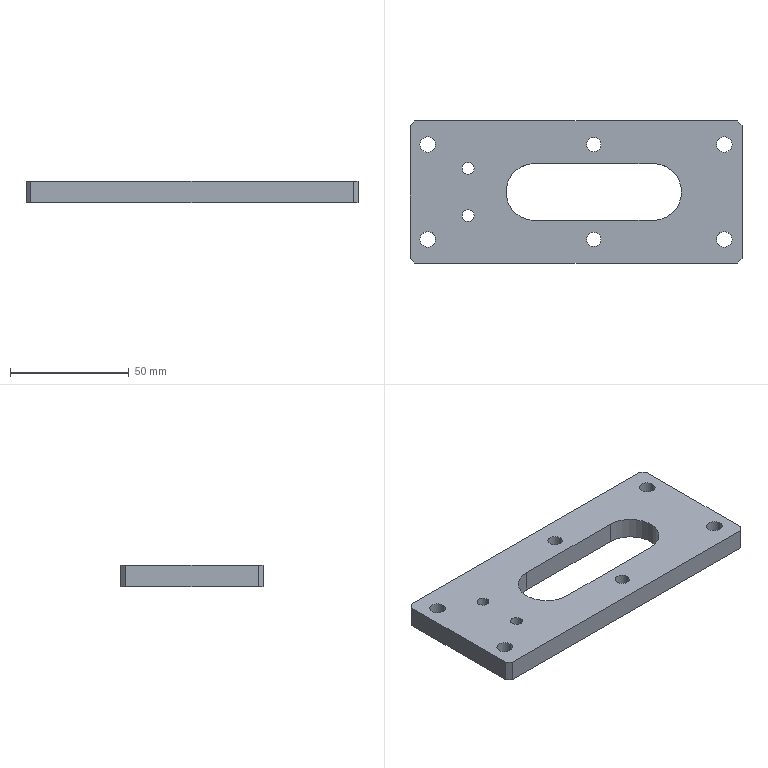Part | STEP file | TNSN20-Y20-F22-Part-14-1 | 1 solid | 30 faces | box 140 x 60 x 9 mm | volume 58562 mm3 | cylinder 18 | plane 12 | commonest cylinder face diameters 6.6 x8 5 x4 6 x4 24 x2
STEP:
#1=CARTESIAN_POINT('',(14042.245,13730.046,0.));
#2=VERTEX_POINT('',#1);
#3=CARTESIAN_POINT('',(14037.245,13730.046,0.));
#4=VERTEX_POINT('',#3);
#5=CARTESIAN_POINT('',(14039.745,13730.046,0.));
#6=DIRECTION('',(0.,0.,-1.));
#7=DIRECTION('',(1.,0.,0.));
#8=AXIS2_PLACEMENT_3D('',#5,#6,#7);
#9=CIRCLE('',#8,2.5);
#10=EDGE_CURVE('',#2,#4,#9,.T.);
#11=ORIENTED_EDGE('',*,*,#10,.T.);
#12=CARTESIAN_POINT('',(14037.245,13730.046,9.));
#13=VERTEX_POINT('',#12);
#14=CARTESIAN_POINT('',(14037.245,13730.046,0.));
#15=DIRECTION('',(0.,0.,1.));
#16=VECTOR('',#15,1000.);
#17=LINE('',#14,#16);
#18=EDGE_CURVE('',#4,#13,#17,.T.);
#19=ORIENTED_EDGE('',*,*,#18,.T.);
#20=CARTESIAN_POINT('',(14042.245,13730.046,9.));
#21=VERTEX_POINT('',#20);
#22=CARTESIAN_POINT('',(14039.745,13730.046,9.));
#23=DIRECTION('',(0.,0.,1.));
#24=DIRECTION('',(-1.,0.,0.));
#25=AXIS2_PLACEMENT_3D('',#22,#23,#24);
#26=CIRCLE('',#25,2.5);
#27=EDGE_CURVE('',#13,#21,#26,.T.);
#28=ORIENTED_EDGE('',*,*,#27,.T.);
#29=CARTESIAN_POINT('',(14042.245,13730.046,0.));
#30=DIRECTION('',(0.,0.,1.));
#31=VECTOR('',#30,1000.);
#32=LINE('',#29,#31);
#33=EDGE_CURVE('',#2,#21,#32,.T.);
#34=ORIENTED_EDGE('',*,*,#33,.F.);
#35=EDGE_LOOP('',(#11,#19,#28,#34));
#36=FACE_OUTER_BOUND('',#35,.T.);
#37=CARTESIAN_POINT('',(14039.745,13730.046,0.));
#38=DIRECTION('',(0.,0.,1.));
#39=DIRECTION('',(1.,0.,0.));
#40=AXIS2_PLACEMENT_3D('',#37,#38,#39);
#41=CYLINDRICAL_SURFACE('',#40,2.5);
#42=ADVANCED_FACE('',(#36),#41,.F.);
#43=CARTESIAN_POINT('',(14042.245,13710.046,0.));
#44=VERTEX_POINT('',#43);
#45=CARTESIAN_POINT('',(14037.245,13710.046,0.));
#46=VERTEX_POINT('',#45);
#47=CARTESIAN_POINT('',(14039.745,13710.046,0.));
#48=DIRECTION('',(0.,0.,-1.));
#49=DIRECTION('',(1.,0.,0.));
#50=AXIS2_PLACEMENT_3D('',#47,#48,#49);
#51=CIRCLE('',#50,2.5);
#52=EDGE_CURVE('',#44,#46,#51,.T.);
#53=ORIENTED_EDGE('',*,*,#52,.T.);
#54=CARTESIAN_POINT('',(14037.245,13710.046,9.));
#55=VERTEX_POINT('',#54);
#56=CARTESIAN_POINT('',(14037.245,13710.046,0.));
#57=DIRECTION('',(0.,0.,1.));
#58=VECTOR('',#57,1000.);
#59=LINE('',#56,#58);
#60=EDGE_CURVE('',#46,#55,#59,.T.);
#61=ORIENTED_EDGE('',*,*,#60,.T.);
#62=CARTESIAN_POINT('',(14042.245,13710.046,9.));
#63=VERTEX_POINT('',#62);
#64=CARTESIAN_POINT('',(14039.745,13710.046,9.));
#65=DIRECTION('',(0.,0.,1.));
#66=DIRECTION('',(-1.,0.,0.));
#67=AXIS2_PLACEMENT_3D('',#64,#65,#66);
#68=CIRCLE('',#67,2.5);
#69=EDGE_CURVE('',#55,#63,#68,.T.);
#70=ORIENTED_EDGE('',*,*,#69,.T.);
#71=CARTESIAN_POINT('',(14042.245,13710.046,0.));
#72=DIRECTION('',(0.,0.,1.));
#73=VECTOR('',#72,1000.);
#74=LINE('',#71,#73);
#75=EDGE_CURVE('',#44,#63,#74,.T.);
#76=ORIENTED_EDGE('',*,*,#75,.F.);
#77=EDGE_LOOP('',(#53,#61,#70,#76));
#78=FACE_OUTER_BOUND('',#77,.T.);
#79=CARTESIAN_POINT('',(14039.745,13710.046,0.));
#80=DIRECTION('',(0.,0.,1.));
#81=DIRECTION('',(1.,0.,0.));
#82=AXIS2_PLACEMENT_3D('',#79,#80,#81);
#83=CYLINDRICAL_SURFACE('',#82,2.5);
#84=ADVANCED_FACE('',(#78),#83,.F.);
#85=CARTESIAN_POINT('',(14095.745,13740.046,0.));
#86=VERTEX_POINT('',#85);
#87=CARTESIAN_POINT('',(14089.745,13740.046,0.));
#88=VERTEX_POINT('',#87);
#89=CARTESIAN_POINT('',(14092.745,13740.046,0.));
#90=DIRECTION('',(0.,0.,-1.));
#91=DIRECTION('',(-1.,0.,0.));
#92=AXIS2_PLACEMENT_3D('',#89,#90,#91);
#93=CIRCLE('',#92,3.);
#94=EDGE_CURVE('',#86,#88,#93,.T.);
#95=ORIENTED_EDGE('',*,*,#94,.T.);
#96=CARTESIAN_POINT('',(14089.745,13740.046,9.));
#97=VERTEX_POINT('',#96);
#98=CARTESIAN_POINT('',(14089.745,13740.046,0.));
#99=DIRECTION('',(0.,0.,1.));
#100=VECTOR('',#99,1000.);
#101=LINE('',#98,#100);
#102=EDGE_CURVE('',#88,#97,#101,.T.);
#103=ORIENTED_EDGE('',*,*,#102,.T.);
#104=CARTESIAN_POINT('',(14095.745,13740.046,9.));
#105=VERTEX_POINT('',#104);
#106=CARTESIAN_POINT('',(14092.745,13740.046,9.));
#107=DIRECTION('',(0.,0.,-1.));
#108=DIRECTION('',(-1.,0.,0.));
#109=AXIS2_PLACEMENT_3D('',#106,#107,#108);
#110=CIRCLE('',#109,3.);
#111=EDGE_CURVE('',#105,#97,#110,.T.);
#112=ORIENTED_EDGE('',*,*,#111,.F.);
#113=CARTESIAN_POINT('',(14095.745,13740.046,0.));
#114=DIRECTION('',(0.,0.,1.));
#115=VECTOR('',#114,1000.);
#116=LINE('',#113,#115);
#117=EDGE_CURVE('',#86,#105,#116,.T.);
#118=ORIENTED_EDGE('',*,*,#117,.F.);
#119=EDGE_LOOP('',(#95,#103,#112,#118));
#120=FACE_OUTER_BOUND('',#119,.T.);
#121=CARTESIAN_POINT('',(14092.745,13740.046,0.));
#122=DIRECTION('',(0.,0.,1.));
#123=DIRECTION('',(1.,0.,0.));
#124=AXIS2_PLACEMENT_3D('',#121,#122,#123);
#125=CYLINDRICAL_SURFACE('',#124,3.);
#126=ADVANCED_FACE('',(#120),#125,.F.);
#127=CARTESIAN_POINT('',(14095.745,13700.046,0.));
#128=VERTEX_POINT('',#127);
#129=CARTESIAN_POINT('',(14089.745,13700.046,0.));
#130=VERTEX_POINT('',#129);
#131=CARTESIAN_POINT('',(14092.745,13700.046,0.));
#132=DIRECTION('',(0.,0.,-1.));
#133=DIRECTION('',(-1.,0.,0.));
#134=AXIS2_PLACEMENT_3D('',#131,#132,#133);
#135=CIRCLE('',#134,3.);
#136=EDGE_CURVE('',#128,#130,#135,.T.);
#137=ORIENTED_EDGE('',*,*,#136,.T.);
#138=CARTESIAN_POINT('',(14089.745,13700.046,9.));
#139=VERTEX_POINT('',#138);
#140=CARTESIAN_POINT('',(14089.745,13700.046,0.));
#141=DIRECTION('',(0.,0.,1.));
#142=VECTOR('',#141,1000.);
#143=LINE('',#140,#142);
#144=EDGE_CURVE('',#130,#139,#143,.T.);
#145=ORIENTED_EDGE('',*,*,#144,.T.);
#146=CARTESIAN_POINT('',(14095.745,13700.046,9.));
#147=VERTEX_POINT('',#146);
#148=CARTESIAN_POINT('',(14092.745,13700.046,9.));
#149=DIRECTION('',(0.,0.,-1.));
#150=DIRECTION('',(-1.,0.,0.));
#151=AXIS2_PLACEMENT_3D('',#148,#149,#150);
#152=CIRCLE('',#151,3.);
#153=EDGE_CURVE('',#147,#139,#152,.T.);
#154=ORIENTED_EDGE('',*,*,#153,.F.);
#155=CARTESIAN_POINT('',(14095.745,13700.046,0.));
#156=DIRECTION('',(0.,0.,1.));
#157=VECTOR('',#156,1000.);
#158=LINE('',#155,#157);
#159=EDGE_CURVE('',#128,#147,#158,.T.);
#160=ORIENTED_EDGE('',*,*,#159,.F.);
#161=EDGE_LOOP('',(#137,#145,#154,#160));
#162=FACE_OUTER_BOUND('',#161,.T.);
#163=CARTESIAN_POINT('',(14092.745,13700.046,0.));
#164=DIRECTION('',(0.,0.,1.));
#165=DIRECTION('',(1.,0.,0.));
#166=AXIS2_PLACEMENT_3D('',#163,#164,#165);
#167=CYLINDRICAL_SURFACE('',#166,3.);
#168=ADVANCED_FACE('',(#162),#167,.F.);
#169=CARTESIAN_POINT('',(14019.445,13700.046,9.));
#170=VERTEX_POINT('',#169);
#171=CARTESIAN_POINT('',(14026.045,13700.046,9.));
#172=VERTEX_POINT('',#171);
#173=CARTESIAN_POINT('',(14022.745,13700.046,9.));
#174=DIRECTION('',(0.,0.,1.));
#175=DIRECTION('',(1.,0.,0.));
#176=AXIS2_PLACEMENT_3D('',#173,#174,#175);
#177=CIRCLE('',#176,3.3);
#178=EDGE_CURVE('',#170,#172,#177,.T.);
#179=ORIENTED_EDGE('',*,*,#178,.T.);
#180=CARTESIAN_POINT('',(14026.045,13700.046,0.));
#181=VERTEX_POINT('',#180);
#182=CARTESIAN_POINT('',(14026.045,13700.046,4.5));
#183=DIRECTION('',(0.,0.,-1.));
#184=VECTOR('',#183,1000.);
#185=LINE('',#182,#184);
#186=EDGE_CURVE('',#172,#181,#185,.T.);
#187=ORIENTED_EDGE('',*,*,#186,.T.);
#188=CARTESIAN_POINT('',(14019.445,13700.046,0.));
#189=VERTEX_POINT('',#188);
#190=CARTESIAN_POINT('',(14022.745,13700.046,0.));
#191=DIRECTION('',(0.,0.,1.));
#192=DIRECTION('',(1.,0.,0.));
#193=AXIS2_PLACEMENT_3D('',#190,#191,#192);
#194=CIRCLE('',#193,3.3);
#195=EDGE_CURVE('',#189,#181,#194,.T.);
#196=ORIENTED_EDGE('',*,*,#195,.F.);
#197=CARTESIAN_POINT('',(14019.445,13700.046,4.5));
#198=DIRECTION('',(0.,0.,-1.));
#199=VECTOR('',#198,1000.);
#200=LINE('',#197,#199);
#201=EDGE_CURVE('',#170,#189,#200,.T.);
#202=ORIENTED_EDGE('',*,*,#201,.F.);
#203=EDGE_LOOP('',(#179,#187,#196,#202));
#204=FACE_OUTER_BOUND('',#203,.T.);
#205=CARTESIAN_POINT('',(14022.745,13700.046,4.5));
#206=DIRECTION('',(0.,0.,-1.));
#207=DIRECTION('',(-1.,0.,0.));
#208=AXIS2_PLACEMENT_3D('',#205,#206,#207);
#209=CYLINDRICAL_SURFACE('',#208,3.3);
#210=ADVANCED_FACE('',(#204),#209,.F.);
#211=CARTESIAN_POINT('',(14019.445,13740.046,9.));
#212=VERTEX_POINT('',#211);
#213=CARTESIAN_POINT('',(14026.045,13740.046,9.));
#214=VERTEX_POINT('',#213);
#215=CARTESIAN_POINT('',(14022.745,13740.046,9.));
#216=DIRECTION('',(0.,0.,1.));
#217=DIRECTION('',(1.,0.,0.));
#218=AXIS2_PLACEMENT_3D('',#215,#216,#217);
#219=CIRCLE('',#218,3.3);
#220=EDGE_CURVE('',#212,#214,#219,.T.);
#221=ORIENTED_EDGE('',*,*,#220,.T.);
#222=CARTESIAN_POINT('',(14026.045,13740.046,0.));
#223=VERTEX_POINT('',#222);
#224=CARTESIAN_POINT('',(14026.045,13740.046,4.5));
#225=DIRECTION('',(0.,0.,-1.));
#226=VECTOR('',#225,1000.);
#227=LINE('',#224,#226);
#228=EDGE_CURVE('',#214,#223,#227,.T.);
#229=ORIENTED_EDGE('',*,*,#228,.T.);
#230=CARTESIAN_POINT('',(14019.445,13740.046,0.));
#231=VERTEX_POINT('',#230);
#232=CARTESIAN_POINT('',(14022.745,13740.046,0.));
#233=DIRECTION('',(0.,0.,1.));
#234=DIRECTION('',(1.,0.,0.));
#235=AXIS2_PLACEMENT_3D('',#232,#233,#234);
#236=CIRCLE('',#235,3.3);
#237=EDGE_CURVE('',#231,#223,#236,.T.);
#238=ORIENTED_EDGE('',*,*,#237,.F.);
#239=CARTESIAN_POINT('',(14019.445,13740.046,4.5));
#240=DIRECTION('',(0.,0.,-1.));
#241=VECTOR('',#240,1000.);
#242=LINE('',#239,#241);
#243=EDGE_CURVE('',#212,#231,#242,.T.);
#244=ORIENTED_EDGE('',*,*,#243,.F.);
#245=EDGE_LOOP('',(#221,#229,#238,#244));
#246=FACE_OUTER_BOUND('',#245,.T.);
#247=CARTESIAN_POINT('',(14022.745,13740.046,4.5));
#248=DIRECTION('',(0.,0.,-1.));
#249=DIRECTION('',(-1.,0.,0.));
#250=AXIS2_PLACEMENT_3D('',#247,#248,#249);
#251=CYLINDRICAL_SURFACE('',#250,3.3);
#252=ADVANCED_FACE('',(#246),#251,.F.);
#253=CARTESIAN_POINT('',(14144.445,13700.046,9.));
#254=VERTEX_POINT('',#253);
#255=CARTESIAN_POINT('',(14151.045,13700.046,9.));
#256=VERTEX_POINT('',#255);
#257=CARTESIAN_POINT('',(14147.745,13700.046,9.));
#258=DIRECTION('',(0.,0.,1.));
#259=DIRECTION('',(1.,0.,0.));
#260=AXIS2_PLACEMENT_3D('',#257,#258,#259);
#261=CIRCLE('',#260,3.3);
#262=EDGE_CURVE('',#254,#256,#261,.T.);
#263=ORIENTED_EDGE('',*,*,#262,.T.);
#264=CARTESIAN_POINT('',(14151.045,13700.046,0.));
#265=VERTEX_POINT('',#264);
#266=CARTESIAN_POINT('',(14151.045,13700.046,4.5));
#267=DIRECTION('',(0.,0.,-1.));
#268=VECTOR('',#267,1000.);
#269=LINE('',#266,#268);
#270=EDGE_CURVE('',#256,#265,#269,.T.);
#271=ORIENTED_EDGE('',*,*,#270,.T.);
#272=CARTESIAN_POINT('',(14144.445,13700.046,0.));
#273=VERTEX_POINT('',#272);
#274=CARTESIAN_POINT('',(14147.745,13700.046,0.));
#275=DIRECTION('',(0.,0.,1.));
#276=DIRECTION('',(1.,0.,0.));
#277=AXIS2_PLACEMENT_3D('',#274,#275,#276);
#278=CIRCLE('',#277,3.3);
#279=EDGE_CURVE('',#273,#265,#278,.T.);
#280=ORIENTED_EDGE('',*,*,#279,.F.);
#281=CARTESIAN_POINT('',(14144.445,13700.046,4.5));
#282=DIRECTION('',(0.,0.,-1.));
#283=VECTOR('',#282,1000.);
#284=LINE('',#281,#283);
#285=EDGE_CURVE('',#254,#273,#284,.T.);
#286=ORIENTED_EDGE('',*,*,#285,.F.);
#287=EDGE_LOOP('',(#263,#271,#280,#286));
#288=FACE_OUTER_BOUND('',#287,.T.);
#289=CARTESIAN_POINT('',(14147.745,13700.046,4.5));
#290=DIRECTION('',(0.,0.,-1.));
#291=DIRECTION('',(-1.,0.,0.));
#292=AXIS2_PLACEMENT_3D('',#289,#290,#291);
#293=CYLINDRICAL_SURFACE('',#292,3.3);
#294=ADVANCED_FACE('',(#288),#293,.F.);
#295=CARTESIAN_POINT('',(14144.445,13740.046,9.));
#296=VERTEX_POINT('',#295);
#297=CARTESIAN_POINT('',(14151.045,13740.046,9.));
#298=VERTEX_POINT('',#297);
#299=CARTESIAN_POINT('',(14147.745,13740.046,9.));
#300=DIRECTION('',(0.,0.,1.));
#301=DIRECTION('',(1.,0.,0.));
#302=AXIS2_PLACEMENT_3D('',#299,#300,#301);
#303=CIRCLE('',#302,3.3);
#304=EDGE_CURVE('',#296,#298,#303,.T.);
#305=ORIENTED_EDGE('',*,*,#304,.T.);
#306=CARTESIAN_POINT('',(14151.045,13740.046,0.));
#307=VERTEX_POINT('',#306);
#308=CARTESIAN_POINT('',(14151.045,13740.046,4.5));
#309=DIRECTION('',(0.,0.,-1.));
#310=VECTOR('',#309,1000.);
#311=LINE('',#308,#310);
#312=EDGE_CURVE('',#298,#307,#311,.T.);
#313=ORIENTED_EDGE('',*,*,#312,.T.);
#314=CARTESIAN_POINT('',(14144.445,13740.046,0.));
#315=VERTEX_POINT('',#314);
#316=CARTESIAN_POINT('',(14147.745,13740.046,0.));
#317=DIRECTION('',(0.,0.,1.));
#318=DIRECTION('',(1.,0.,0.));
#319=AXIS2_PLACEMENT_3D('',#316,#317,#318);
#320=CIRCLE('',#319,3.3);
#321=EDGE_CURVE('',#315,#307,#320,.T.);
#322=ORIENTED_EDGE('',*,*,#321,.F.);
#323=CARTESIAN_POINT('',(14144.445,13740.046,4.5));
#324=DIRECTION('',(0.,0.,-1.));
#325=VECTOR('',#324,1000.);
#326=LINE('',#323,#325);
#327=EDGE_CURVE('',#296,#315,#326,.T.);
#328=ORIENTED_EDGE('',*,*,#327,.F.);
#329=EDGE_LOOP('',(#305,#313,#322,#328));
#330=FACE_OUTER_BOUND('',#329,.T.);
#331=CARTESIAN_POINT('',(14147.745,13740.046,4.5));
#332=DIRECTION('',(0.,0.,-1.));
#333=DIRECTION('',(-1.,0.,0.));
#334=AXIS2_PLACEMENT_3D('',#331,#332,#333);
#335=CYLINDRICAL_SURFACE('',#334,3.3);
#336=ADVANCED_FACE('',(#330),#335,.F.);
#337=CARTESIAN_POINT('',(14015.245,13748.046,0.));
#338=VERTEX_POINT('',#337);
#339=CARTESIAN_POINT('',(14015.245,13692.046,0.));
#340=VERTEX_POINT('',#339);
#341=CARTESIAN_POINT('',(14015.245,13748.046,0.));
#342=DIRECTION('',(0.,-1.,0.));
#343=VECTOR('',#342,1000.);
#344=LINE('',#341,#343);
#345=EDGE_CURVE('',#338,#340,#344,.T.);
#346=ORIENTED_EDGE('',*,*,#345,.T.);
#347=CARTESIAN_POINT('',(14015.245,13692.046,9.));
#348=VERTEX_POINT('',#347);
#349=CARTESIAN_POINT('',(14015.245,13692.046,9.));
#350=DIRECTION('',(0.,0.,-1.));
#351=VECTOR('',#350,1000.);
#352=LINE('',#349,#351);
#353=EDGE_CURVE('',#348,#340,#352,.T.);
#354=ORIENTED_EDGE('',*,*,#353,.F.);
#355=CARTESIAN_POINT('',(14015.245,13748.046,9.));
#356=VERTEX_POINT('',#355);
#357=CARTESIAN_POINT('',(14015.245,13748.046,9.));
#358=DIRECTION('',(0.,-1.,0.));
#359=VECTOR('',#358,1000.);
#360=LINE('',#357,#359);
#361=EDGE_CURVE('',#356,#348,#360,.T.);
#362=ORIENTED_EDGE('',*,*,#361,.F.);
#363=CARTESIAN_POINT('',(14015.245,13748.046,9.));
#364=DIRECTION('',(0.,0.,-1.));
#365=VECTOR('',#364,1000.);
#366=LINE('',#363,#365);
#367=EDGE_CURVE('',#356,#338,#366,.T.);
#368=ORIENTED_EDGE('',*,*,#367,.T.);
#369=EDGE_LOOP('',(#346,#354,#362,#368));
#370=FACE_OUTER_BOUND('',#369,.T.);
#371=CARTESIAN_POINT('',(14015.245,13677.507,47.039));
#372=DIRECTION('',(1.,0.,0.));
#373=DIRECTION('',(0.,0.,-1.));
#374=AXIS2_PLACEMENT_3D('',#371,#372,#373);
#375=PLANE('',#374);
#376=ADVANCED_FACE('',(#370),#375,.F.);
#377=CARTESIAN_POINT('',(14017.245,13690.046,0.));
#378=VERTEX_POINT('',#377);
#379=CARTESIAN_POINT('',(14015.245,13692.046,0.));
#380=DIRECTION('',(0.7071,-0.7071,0.));
#381=VECTOR('',#380,1000.);
#382=LINE('',#379,#381);
#383=EDGE_CURVE('',#340,#378,#382,.T.);
#384=ORIENTED_EDGE('',*,*,#383,.T.);
#385=CARTESIAN_POINT('',(14017.245,13690.046,9.));
#386=VERTEX_POINT('',#385);
#387=CARTESIAN_POINT('',(14017.245,13690.046,9.));
#388=DIRECTION('',(0.,0.,-1.));
#389=VECTOR('',#388,1000.);
#390=LINE('',#387,#389);
#391=EDGE_CURVE('',#386,#378,#390,.T.);
#392=ORIENTED_EDGE('',*,*,#391,.F.);
#393=CARTESIAN_POINT('',(14015.245,13692.046,9.));
#394=DIRECTION('',(0.7071,-0.7071,0.));
#395=VECTOR('',#394,1000.);
#396=LINE('',#393,#395);
#397=EDGE_CURVE('',#348,#386,#396,.T.);
#398=ORIENTED_EDGE('',*,*,#397,.F.);
#399=ORIENTED_EDGE('',*,*,#353,.T.);
#400=EDGE_LOOP('',(#384,#392,#398,#399));
#401=FACE_OUTER_BOUND('',#400,.T.);
#402=CARTESIAN_POINT('',(14021.248,13686.043,-2.575));
#403=DIRECTION('',(0.7071,0.7071,0.));
#404=DIRECTION('',(-0.7071,0.7071,0.));
#405=AXIS2_PLACEMENT_3D('',#402,#403,#404);
#406=PLANE('',#405);
#407=ADVANCED_FACE('',(#401),#406,.F.);
#408=CARTESIAN_POINT('',(14153.245,13690.046,0.));
#409=VERTEX_POINT('',#408);
#410=CARTESIAN_POINT('',(14017.245,13690.046,0.));
#411=DIRECTION('',(1.,0.,0.));
#412=VECTOR('',#411,1000.);
#413=LINE('',#410,#412);
#414=EDGE_CURVE('',#378,#409,#413,.T.);
#415=ORIENTED_EDGE('',*,*,#414,.T.);
#416=CARTESIAN_POINT('',(14153.245,13690.046,9.));
#417=VERTEX_POINT('',#416);
#418=CARTESIAN_POINT('',(14153.245,13690.046,9.));
#419=DIRECTION('',(0.,0.,-1.));
#420=VECTOR('',#419,1000.);
#421=LINE('',#418,#420);
#422=EDGE_CURVE('',#417,#409,#421,.T.);
#423=ORIENTED_EDGE('',*,*,#422,.F.);
#424=CARTESIAN_POINT('',(14017.245,13690.046,9.));
#425=DIRECTION('',(1.,0.,0.));
#426=VECTOR('',#425,1000.);
#427=LINE('',#424,#426);
#428=EDGE_CURVE('',#386,#417,#427,.T.);
#429=ORIENTED_EDGE('',*,*,#428,.F.);
#430=ORIENTED_EDGE('',*,*,#391,.T.);
#431=EDGE_LOOP('',(#415,#423,#429,#430));
#432=FACE_OUTER_BOUND('',#431,.T.);
#433=CARTESIAN_POINT('',(13983.022,13690.046,-97.723));
#434=DIRECTION('',(0.,1.,0.));
#435=DIRECTION('',(0.,0.,1.));
#436=AXIS2_PLACEMENT_3D('',#433,#434,#435);
#437=PLANE('',#436);
#438=ADVANCED_FACE('',(#432),#437,.F.);
#439=CARTESIAN_POINT('',(14155.245,13692.046,0.));
#440=VERTEX_POINT('',#439);
#441=CARTESIAN_POINT('',(14153.245,13690.046,0.));
#442=DIRECTION('',(0.7071,0.7071,0.));
#443=VECTOR('',#442,1000.);
#444=LINE('',#441,#443);
#445=EDGE_CURVE('',#409,#440,#444,.T.);
#446=ORIENTED_EDGE('',*,*,#445,.T.);
#447=CARTESIAN_POINT('',(14155.245,13692.046,9.));
#448=VERTEX_POINT('',#447);
#449=CARTESIAN_POINT('',(14155.245,13692.046,9.));
#450=DIRECTION('',(0.,0.,-1.));
#451=VECTOR('',#450,1000.);
#452=LINE('',#449,#451);
#453=EDGE_CURVE('',#448,#440,#452,.T.);
#454=ORIENTED_EDGE('',*,*,#453,.F.);
#455=CARTESIAN_POINT('',(14153.245,13690.046,9.));
#456=DIRECTION('',(0.7071,0.7071,0.));
#457=VECTOR('',#456,1000.);
#458=LINE('',#455,#457);
#459=EDGE_CURVE('',#417,#448,#458,.T.);
#460=ORIENTED_EDGE('',*,*,#459,.F.);
#461=ORIENTED_EDGE('',*,*,#422,.T.);
#462=EDGE_LOOP('',(#446,#454,#460,#461));
#463=FACE_OUTER_BOUND('',#462,.T.);
#464=CARTESIAN_POINT('',(14159.248,13696.049,-2.575));
#465=DIRECTION('',(-0.7071,0.7071,0.));
#466=DIRECTION('',(-0.7071,-0.7071,0.));
#467=AXIS2_PLACEMENT_3D('',#464,#465,#466);
#468=PLANE('',#467);
#469=ADVANCED_FACE('',(#463),#468,.F.);
#470=CARTESIAN_POINT('',(14155.245,13748.046,0.));
#471=VERTEX_POINT('',#470);
#472=CARTESIAN_POINT('',(14155.245,13692.046,0.));
#473=DIRECTION('',(0.,1.,0.));
#474=VECTOR('',#473,1000.);
#475=LINE('',#472,#474);
#476=EDGE_CURVE('',#440,#471,#475,.T.);
#477=ORIENTED_EDGE('',*,*,#476,.T.);
#478=CARTESIAN_POINT('',(14155.245,13748.046,9.));
#479=VERTEX_POINT('',#478);
#480=CARTESIAN_POINT('',(14155.245,13748.046,9.));
#481=DIRECTION('',(0.,0.,-1.));
#482=VECTOR('',#481,1000.);
#483=LINE('',#480,#482);
#484=EDGE_CURVE('',#479,#471,#483,.T.);
#485=ORIENTED_EDGE('',*,*,#484,.F.);
#486=CARTESIAN_POINT('',(14155.245,13692.046,9.));
#487=DIRECTION('',(0.,1.,0.));
#488=VECTOR('',#487,1000.);
#489=LINE('',#486,#488);
#490=EDGE_CURVE('',#448,#479,#489,.T.);
#491=ORIENTED_EDGE('',*,*,#490,.F.);
#492=ORIENTED_EDGE('',*,*,#453,.T.);
#493=EDGE_LOOP('',(#477,#485,#491,#492));
#494=FACE_OUTER_BOUND('',#493,.T.);
#495=CARTESIAN_POINT('',(14155.245,13677.507,-38.039));
#496=DIRECTION('',(-1.,0.,0.));
#497=DIRECTION('',(0.,0.,1.));
#498=AXIS2_PLACEMENT_3D('',#495,#496,#497);
#499=PLANE('',#498);
#500=ADVANCED_FACE('',(#494),#499,.F.);
#501=CARTESIAN_POINT('',(14153.245,13750.046,0.));
#502=VERTEX_POINT('',#501);
#503=CARTESIAN_POINT('',(14155.245,13748.046,0.));
#504=DIRECTION('',(-0.7071,0.7071,0.));
#505=VECTOR('',#504,1000.);
#506=LINE('',#503,#505);
#507=EDGE_CURVE('',#471,#502,#506,.T.);
#508=ORIENTED_EDGE('',*,*,#507,.T.);
#509=CARTESIAN_POINT('',(14153.245,13750.046,9.));
#510=VERTEX_POINT('',#509);
#511=CARTESIAN_POINT('',(14153.245,13750.046,9.));
#512=DIRECTION('',(0.,0.,-1.));
#513=VECTOR('',#512,1000.);
#514=LINE('',#511,#513);
#515=EDGE_CURVE('',#510,#502,#514,.T.);
#516=ORIENTED_EDGE('',*,*,#515,.F.);
#517=CARTESIAN_POINT('',(14155.245,13748.046,9.));
#518=DIRECTION('',(-0.7071,0.7071,0.));
#519=VECTOR('',#518,1000.);
#520=LINE('',#517,#519);
#521=EDGE_CURVE('',#479,#510,#520,.T.);
#522=ORIENTED_EDGE('',*,*,#521,.F.);
#523=ORIENTED_EDGE('',*,*,#484,.T.);
#524=EDGE_LOOP('',(#508,#516,#522,#523));
#525=FACE_OUTER_BOUND('',#524,.T.);
#526=CARTESIAN_POINT('',(14149.242,13754.049,-2.575));
#527=DIRECTION('',(-0.7071,-0.7071,0.));
#528=DIRECTION('',(0.7071,-0.7071,0.));
#529=AXIS2_PLACEMENT_3D('',#526,#527,#528);
#530=PLANE('',#529);
#531=ADVANCED_FACE('',(#525),#530,.F.);
#532=CARTESIAN_POINT('',(14017.245,13750.046,0.));
#533=VERTEX_POINT('',#532);
#534=CARTESIAN_POINT('',(14153.245,13750.046,0.));
#535=DIRECTION('',(-1.,0.,0.));
#536=VECTOR('',#535,1000.);
#537=LINE('',#534,#536);
#538=EDGE_CURVE('',#502,#533,#537,.T.);
#539=ORIENTED_EDGE('',*,*,#538,.T.);
#540=CARTESIAN_POINT('',(14017.245,13750.046,9.));
#541=VERTEX_POINT('',#540);
#542=CARTESIAN_POINT('',(14017.245,13750.046,9.));
#543=DIRECTION('',(0.,0.,-1.));
#544=VECTOR('',#543,1000.);
#545=LINE('',#542,#544);
#546=EDGE_CURVE('',#541,#533,#545,.T.);
#547=ORIENTED_EDGE('',*,*,#546,.F.);
#548=CARTESIAN_POINT('',(14153.245,13750.046,9.));
#549=DIRECTION('',(-1.,0.,0.));
#550=VECTOR('',#549,1000.);
#551=LINE('',#548,#550);
#552=EDGE_CURVE('',#510,#541,#551,.T.);
#553=ORIENTED_EDGE('',*,*,#552,.F.);
#554=ORIENTED_EDGE('',*,*,#515,.T.);
#555=EDGE_LOOP('',(#539,#547,#553,#554));
#556=FACE_OUTER_BOUND('',#555,.T.);
#557=CARTESIAN_POINT('',(13983.022,13750.046,106.723));
#558=DIRECTION('',(0.,-1.,0.));
#559=DIRECTION('',(0.,0.,-1.));
#560=AXIS2_PLACEMENT_3D('',#557,#558,#559);
#561=PLANE('',#560);
#562=ADVANCED_FACE('',(#556),#561,.F.);
#563=CARTESIAN_POINT('',(14117.745,13732.046,0.));
#564=VERTEX_POINT('',#563);
#565=CARTESIAN_POINT('',(14067.745,13732.046,0.));
#566=VERTEX_POINT('',#565);
#567=CARTESIAN_POINT('',(14117.745,13732.046,0.));
#568=DIRECTION('',(-1.,0.,0.));
#569=VECTOR('',#568,1000.);
#570=LINE('',#567,#569);
#571=EDGE_CURVE('',#564,#566,#570,.T.);
#572=ORIENTED_EDGE('',*,*,#571,.F.);
#573=CARTESIAN_POINT('',(14117.745,13732.046,9.));
#574=VERTEX_POINT('',#573);
#575=CARTESIAN_POINT('',(14117.745,13732.046,9.));
#576=DIRECTION('',(0.,0.,-1.));
#577=VECTOR('',#576,1000.);
#578=LINE('',#575,#577);
#579=EDGE_CURVE('',#574,#564,#578,.T.);
#580=ORIENTED_EDGE('',*,*,#579,.F.);
#581=CARTESIAN_POINT('',(14067.745,13732.046,9.));
#582=VERTEX_POINT('',#581);
#583=CARTESIAN_POINT('',(14117.745,13732.046,9.));
#584=DIRECTION('',(-1.,0.,0.));
#585=VECTOR('',#584,1000.);
#586=LINE('',#583,#585);
#587=EDGE_CURVE('',#574,#582,#586,.T.);
#588=ORIENTED_EDGE('',*,*,#587,.T.);
#589=CARTESIAN_POINT('',(14067.745,13732.046,9.));
#590=DIRECTION('',(0.,0.,-1.));
#591=VECTOR('',#590,1000.);
#592=LINE('',#589,#591);
#593=EDGE_CURVE('',#582,#566,#592,.T.);
#594=ORIENTED_EDGE('',*,*,#593,.T.);
#595=EDGE_LOOP('',(#572,#580,#588,#594));
#596=FACE_OUTER_BOUND('',#595,.T.);
#597=CARTESIAN_POINT('',(14054.642,13732.046,42.603));
#598=DIRECTION('',(0.,-1.,0.));
#599=DIRECTION('',(0.,0.,-1.));
#600=AXIS2_PLACEMENT_3D('',#597,#598,#599);
#601=PLANE('',#600);
#602=ADVANCED_FACE('',(#596),#601,.T.);
#603=CARTESIAN_POINT('',(14117.745,13708.046,0.));
#604=VERTEX_POINT('',#603);
#605=CARTESIAN_POINT('',(14117.745,13720.046,0.));
#606=DIRECTION('',(0.,0.,1.));
#607=DIRECTION('',(0.,-1.,0.));
#608=AXIS2_PLACEMENT_3D('',#605,#606,#607);
#609=CIRCLE('',#608,12.);
#610=EDGE_CURVE('',#604,#564,#609,.T.);
#611=ORIENTED_EDGE('',*,*,#610,.F.);
#612=CARTESIAN_POINT('',(14117.745,13708.046,9.));
#613=VERTEX_POINT('',#612);
#614=CARTESIAN_POINT('',(14117.745,13708.046,9.));
#615=DIRECTION('',(0.,0.,-1.));
#616=VECTOR('',#615,1000.);
#617=LINE('',#614,#616);
#618=EDGE_CURVE('',#613,#604,#617,.T.);
#619=ORIENTED_EDGE('',*,*,#618,.F.);
#620=CARTESIAN_POINT('',(14117.745,13720.046,9.));
#621=DIRECTION('',(0.,0.,1.));
#622=DIRECTION('',(0.,-1.,0.));
#623=AXIS2_PLACEMENT_3D('',#620,#621,#622);
#624=CIRCLE('',#623,12.);
#625=EDGE_CURVE('',#613,#574,#624,.T.);
#626=ORIENTED_EDGE('',*,*,#625,.T.);
#627=ORIENTED_EDGE('',*,*,#579,.T.);
#628=EDGE_LOOP('',(#611,#619,#626,#627));
#629=FACE_OUTER_BOUND('',#628,.T.);
#630=CARTESIAN_POINT('',(14117.745,13720.046,4.5));
#631=DIRECTION('',(0.,0.,-1.));
#632=DIRECTION('',(-1.,0.,0.));
#633=AXIS2_PLACEMENT_3D('',#630,#631,#632);
#634=CYLINDRICAL_SURFACE('',#633,12.);
#635=ADVANCED_FACE('',(#629),#634,.F.);
#636=CARTESIAN_POINT('',(14067.745,13708.046,0.));
#637=VERTEX_POINT('',#636);
#638=CARTESIAN_POINT('',(14067.745,13708.046,0.));
#639=DIRECTION('',(1.,0.,0.));
#640=VECTOR('',#639,1000.);
#641=LINE('',#638,#640);
#642=EDGE_CURVE('',#637,#604,#641,.T.);
#643=ORIENTED_EDGE('',*,*,#642,.F.);
#644=CARTESIAN_POINT('',(14067.745,13708.046,9.));
#645=VERTEX_POINT('',#644);
#646=CARTESIAN_POINT('',(14067.745,13708.046,9.));
#647=DIRECTION('',(0.,0.,-1.));
#648=VECTOR('',#647,1000.);
#649=LINE('',#646,#648);
#650=EDGE_CURVE('',#645,#637,#649,.T.);
#651=ORIENTED_EDGE('',*,*,#650,.F.);
#652=CARTESIAN_POINT('',(14067.745,13708.046,9.));
#653=DIRECTION('',(1.,0.,0.));
#654=VECTOR('',#653,1000.);
#655=LINE('',#652,#654);
#656=EDGE_CURVE('',#645,#613,#655,.T.);
#657=ORIENTED_EDGE('',*,*,#656,.T.);
#658=ORIENTED_EDGE('',*,*,#618,.T.);
#659=EDGE_LOOP('',(#643,#651,#657,#658));
#660=FACE_OUTER_BOUND('',#659,.T.);
#661=CARTESIAN_POINT('',(14054.642,13708.046,-33.603));
#662=DIRECTION('',(0.,1.,0.));
#663=DIRECTION('',(0.,0.,1.));
#664=AXIS2_PLACEMENT_3D('',#661,#662,#663);
#665=PLANE('',#664);
#666=ADVANCED_FACE('',(#660),#665,.T.);
#667=CARTESIAN_POINT('',(14067.745,13720.046,0.));
#668=DIRECTION('',(0.,0.,1.));
#669=DIRECTION('',(0.,1.,0.));
#670=AXIS2_PLACEMENT_3D('',#667,#668,#669);
#671=CIRCLE('',#670,12.);
#672=EDGE_CURVE('',#566,#637,#671,.T.);
#673=ORIENTED_EDGE('',*,*,#672,.F.);
#674=ORIENTED_EDGE('',*,*,#593,.F.);
#675=CARTESIAN_POINT('',(14067.745,13720.046,9.));
#676=DIRECTION('',(0.,0.,1.));
#677=DIRECTION('',(0.,1.,0.));
#678=AXIS2_PLACEMENT_3D('',#675,#676,#677);
#679=CIRCLE('',#678,12.);
#680=EDGE_CURVE('',#582,#645,#679,.T.);
#681=ORIENTED_EDGE('',*,*,#680,.T.);
#682=ORIENTED_EDGE('',*,*,#650,.T.);
#683=EDGE_LOOP('',(#673,#674,#681,#682));
#684=FACE_OUTER_BOUND('',#683,.T.);
#685=CARTESIAN_POINT('',(14067.745,13720.046,4.5));
#686=DIRECTION('',(0.,0.,-1.));
#687=DIRECTION('',(1.,0.,0.));
#688=AXIS2_PLACEMENT_3D('',#685,#686,#687);
#689=CYLINDRICAL_SURFACE('',#688,12.);
#690=ADVANCED_FACE('',(#684),#689,.F.);
#691=CARTESIAN_POINT('',(14017.245,13750.046,0.));
#692=DIRECTION('',(-0.7071,-0.7071,0.));
#693=VECTOR('',#692,1000.);
#694=LINE('',#691,#693);
#695=EDGE_CURVE('',#533,#338,#694,.T.);
#696=ORIENTED_EDGE('',*,*,#695,.T.);
#697=ORIENTED_EDGE('',*,*,#367,.F.);
#698=CARTESIAN_POINT('',(14017.245,13750.046,9.));
#699=DIRECTION('',(-0.7071,-0.7071,0.));
#700=VECTOR('',#699,1000.);
#701=LINE('',#698,#700);
#702=EDGE_CURVE('',#541,#356,#701,.T.);
#703=ORIENTED_EDGE('',*,*,#702,.F.);
#704=ORIENTED_EDGE('',*,*,#546,.T.);
#705=EDGE_LOOP('',(#696,#697,#703,#704));
#706=FACE_OUTER_BOUND('',#705,.T.);
#707=CARTESIAN_POINT('',(14011.242,13744.043,-2.575));
#708=DIRECTION('',(0.7071,-0.7071,0.));
#709=DIRECTION('',(0.7071,0.7071,0.));
#710=AXIS2_PLACEMENT_3D('',#707,#708,#709);
#711=PLANE('',#710);
#712=ADVANCED_FACE('',(#706),#711,.F.);
#713=ORIENTED_EDGE('',*,*,#361,.T.);
#714=ORIENTED_EDGE('',*,*,#397,.T.);
#715=ORIENTED_EDGE('',*,*,#428,.T.);
#716=ORIENTED_EDGE('',*,*,#459,.T.);
#717=ORIENTED_EDGE('',*,*,#490,.T.);
#718=ORIENTED_EDGE('',*,*,#521,.T.);
#719=ORIENTED_EDGE('',*,*,#552,.T.);
#720=ORIENTED_EDGE('',*,*,#702,.T.);
#721=EDGE_LOOP('',(#713,#714,#715,#716,#717,#718,#719,#720));
#722=FACE_OUTER_BOUND('',#721,.T.);
#723=ORIENTED_EDGE('',*,*,#153,.T.);
#724=CARTESIAN_POINT('',(14092.745,13700.046,9.));
#725=DIRECTION('',(0.,0.,-1.));
#726=DIRECTION('',(-1.,0.,0.));
#727=AXIS2_PLACEMENT_3D('',#724,#725,#726);
#728=CIRCLE('',#727,3.);
#729=EDGE_CURVE('',#139,#147,#728,.T.);
#730=ORIENTED_EDGE('',*,*,#729,.T.);
#731=EDGE_LOOP('',(#723,#730));
#732=FACE_BOUND('',#731,.T.);
#733=ORIENTED_EDGE('',*,*,#111,.T.);
#734=CARTESIAN_POINT('',(14092.745,13740.046,9.));
#735=DIRECTION('',(0.,0.,-1.));
#736=DIRECTION('',(-1.,0.,0.));
#737=AXIS2_PLACEMENT_3D('',#734,#735,#736);
#738=CIRCLE('',#737,3.);
#739=EDGE_CURVE('',#97,#105,#738,.T.);
#740=ORIENTED_EDGE('',*,*,#739,.T.);
#741=EDGE_LOOP('',(#733,#740));
#742=FACE_BOUND('',#741,.T.);
#743=CARTESIAN_POINT('',(14039.745,13710.046,9.));
#744=DIRECTION('',(0.,0.,1.));
#745=DIRECTION('',(-1.,0.,0.));
#746=AXIS2_PLACEMENT_3D('',#743,#744,#745);
#747=CIRCLE('',#746,2.5);
#748=EDGE_CURVE('',#63,#55,#747,.T.);
#749=ORIENTED_EDGE('',*,*,#748,.F.);
#750=ORIENTED_EDGE('',*,*,#69,.F.);
#751=EDGE_LOOP('',(#749,#750));
#752=FACE_BOUND('',#751,.T.);
#753=CARTESIAN_POINT('',(14039.745,13730.046,9.));
#754=DIRECTION('',(0.,0.,1.));
#755=DIRECTION('',(-1.,0.,0.));
#756=AXIS2_PLACEMENT_3D('',#753,#754,#755);
#757=CIRCLE('',#756,2.5);
#758=EDGE_CURVE('',#21,#13,#757,.T.);
#759=ORIENTED_EDGE('',*,*,#758,.F.);
#760=ORIENTED_EDGE('',*,*,#27,.F.);
#761=EDGE_LOOP('',(#759,#760));
#762=FACE_BOUND('',#761,.T.);
#763=ORIENTED_EDGE('',*,*,#178,.F.);
#764=CARTESIAN_POINT('',(14022.745,13700.046,9.));
#765=DIRECTION('',(0.,0.,1.));
#766=DIRECTION('',(1.,0.,0.));
#767=AXIS2_PLACEMENT_3D('',#764,#765,#766);
#768=CIRCLE('',#767,3.3);
#769=EDGE_CURVE('',#172,#170,#768,.T.);
#770=ORIENTED_EDGE('',*,*,#769,.F.);
#771=EDGE_LOOP('',(#763,#770));
#772=FACE_BOUND('',#771,.T.);
#773=ORIENTED_EDGE('',*,*,#220,.F.);
#774=CARTESIAN_POINT('',(14022.745,13740.046,9.));
#775=DIRECTION('',(0.,0.,1.));
#776=DIRECTION('',(1.,0.,0.));
#777=AXIS2_PLACEMENT_3D('',#774,#775,#776);
#778=CIRCLE('',#777,3.3);
#779=EDGE_CURVE('',#214,#212,#778,.T.);
#780=ORIENTED_EDGE('',*,*,#779,.F.);
#781=EDGE_LOOP('',(#773,#780));
#782=FACE_BOUND('',#781,.T.);
#783=ORIENTED_EDGE('',*,*,#587,.F.);
#784=ORIENTED_EDGE('',*,*,#625,.F.);
#785=ORIENTED_EDGE('',*,*,#656,.F.);
#786=ORIENTED_EDGE('',*,*,#680,.F.);
#787=EDGE_LOOP('',(#783,#784,#785,#786));
#788=FACE_BOUND('',#787,.T.);
#789=ORIENTED_EDGE('',*,*,#262,.F.);
#790=CARTESIAN_POINT('',(14147.745,13700.046,9.));
#791=DIRECTION('',(0.,0.,1.));
#792=DIRECTION('',(1.,0.,0.));
#793=AXIS2_PLACEMENT_3D('',#790,#791,#792);
#794=CIRCLE('',#793,3.3);
#795=EDGE_CURVE('',#256,#254,#794,.T.);
#796=ORIENTED_EDGE('',*,*,#795,.F.);
#797=EDGE_LOOP('',(#789,#796));
#798=FACE_BOUND('',#797,.T.);
#799=ORIENTED_EDGE('',*,*,#304,.F.);
#800=CARTESIAN_POINT('',(14147.745,13740.046,9.));
#801=DIRECTION('',(0.,0.,1.));
#802=DIRECTION('',(1.,0.,0.));
#803=AXIS2_PLACEMENT_3D('',#800,#801,#802);
#804=CIRCLE('',#803,3.3);
#805=EDGE_CURVE('',#298,#296,#804,.T.);
#806=ORIENTED_EDGE('',*,*,#805,.F.);
#807=EDGE_LOOP('',(#799,#806));
#808=FACE_BOUND('',#807,.T.);
#809=CARTESIAN_POINT('',(13971.008,13605.81,9.));
#810=DIRECTION('',(0.,0.,1.));
#811=DIRECTION('',(1.,0.,0.));
#812=AXIS2_PLACEMENT_3D('',#809,#810,#811);
#813=PLANE('',#812);
#814=ADVANCED_FACE('',(#722,#732,#742,#752,#762,#772,#782,#788,#798,#808),#813,.T.);
#815=ORIENTED_EDGE('',*,*,#345,.F.);
#816=ORIENTED_EDGE('',*,*,#695,.F.);
#817=ORIENTED_EDGE('',*,*,#538,.F.);
#818=ORIENTED_EDGE('',*,*,#507,.F.);
#819=ORIENTED_EDGE('',*,*,#476,.F.);
#820=ORIENTED_EDGE('',*,*,#445,.F.);
#821=ORIENTED_EDGE('',*,*,#414,.F.);
#822=ORIENTED_EDGE('',*,*,#383,.F.);
#823=EDGE_LOOP('',(#815,#816,#817,#818,#819,#820,#821,#822));
#824=FACE_OUTER_BOUND('',#823,.T.);
#825=ORIENTED_EDGE('',*,*,#136,.F.);
#826=CARTESIAN_POINT('',(14092.745,13700.046,0.));
#827=DIRECTION('',(0.,0.,-1.));
#828=DIRECTION('',(-1.,0.,0.));
#829=AXIS2_PLACEMENT_3D('',#826,#827,#828);
#830=CIRCLE('',#829,3.);
#831=EDGE_CURVE('',#130,#128,#830,.T.);
#832=ORIENTED_EDGE('',*,*,#831,.F.);
#833=EDGE_LOOP('',(#825,#832));
#834=FACE_BOUND('',#833,.T.);
#835=ORIENTED_EDGE('',*,*,#94,.F.);
#836=CARTESIAN_POINT('',(14092.745,13740.046,0.));
#837=DIRECTION('',(0.,0.,-1.));
#838=DIRECTION('',(-1.,0.,0.));
#839=AXIS2_PLACEMENT_3D('',#836,#837,#838);
#840=CIRCLE('',#839,3.);
#841=EDGE_CURVE('',#88,#86,#840,.T.);
#842=ORIENTED_EDGE('',*,*,#841,.F.);
#843=EDGE_LOOP('',(#835,#842));
#844=FACE_BOUND('',#843,.T.);
#845=ORIENTED_EDGE('',*,*,#52,.F.);
#846=CARTESIAN_POINT('',(14039.745,13710.046,0.));
#847=DIRECTION('',(0.,0.,-1.));
#848=DIRECTION('',(1.,0.,0.));
#849=AXIS2_PLACEMENT_3D('',#846,#847,#848);
#850=CIRCLE('',#849,2.5);
#851=EDGE_CURVE('',#46,#44,#850,.T.);
#852=ORIENTED_EDGE('',*,*,#851,.F.);
#853=EDGE_LOOP('',(#845,#852));
#854=FACE_BOUND('',#853,.T.);
#855=ORIENTED_EDGE('',*,*,#10,.F.);
#856=CARTESIAN_POINT('',(14039.745,13730.046,0.));
#857=DIRECTION('',(0.,0.,-1.));
#858=DIRECTION('',(1.,0.,0.));
#859=AXIS2_PLACEMENT_3D('',#856,#857,#858);
#860=CIRCLE('',#859,2.5);
#861=EDGE_CURVE('',#4,#2,#860,.T.);
#862=ORIENTED_EDGE('',*,*,#861,.F.);
#863=EDGE_LOOP('',(#855,#862));
#864=FACE_BOUND('',#863,.T.);
#865=ORIENTED_EDGE('',*,*,#195,.T.);
#866=CARTESIAN_POINT('',(14022.745,13700.046,0.));
#867=DIRECTION('',(0.,0.,1.));
#868=DIRECTION('',(1.,0.,0.));
#869=AXIS2_PLACEMENT_3D('',#866,#867,#868);
#870=CIRCLE('',#869,3.3);
#871=EDGE_CURVE('',#181,#189,#870,.T.);
#872=ORIENTED_EDGE('',*,*,#871,.T.);
#873=EDGE_LOOP('',(#865,#872));
#874=FACE_BOUND('',#873,.T.);
#875=ORIENTED_EDGE('',*,*,#237,.T.);
#876=CARTESIAN_POINT('',(14022.745,13740.046,0.));
#877=DIRECTION('',(0.,0.,1.));
#878=DIRECTION('',(1.,0.,0.));
#879=AXIS2_PLACEMENT_3D('',#876,#877,#878);
#880=CIRCLE('',#879,3.3);
#881=EDGE_CURVE('',#223,#231,#880,.T.);
#882=ORIENTED_EDGE('',*,*,#881,.T.);
#883=EDGE_LOOP('',(#875,#882));
#884=FACE_BOUND('',#883,.T.);
#885=ORIENTED_EDGE('',*,*,#571,.T.);
#886=ORIENTED_EDGE('',*,*,#672,.T.);
#887=ORIENTED_EDGE('',*,*,#642,.T.);
#888=ORIENTED_EDGE('',*,*,#610,.T.);
#889=EDGE_LOOP('',(#885,#886,#887,#888));
#890=FACE_BOUND('',#889,.T.);
#891=ORIENTED_EDGE('',*,*,#279,.T.);
#892=CARTESIAN_POINT('',(14147.745,13700.046,0.));
#893=DIRECTION('',(0.,0.,1.));
#894=DIRECTION('',(1.,0.,0.));
#895=AXIS2_PLACEMENT_3D('',#892,#893,#894);
#896=CIRCLE('',#895,3.3);
#897=EDGE_CURVE('',#265,#273,#896,.T.);
#898=ORIENTED_EDGE('',*,*,#897,.T.);
#899=EDGE_LOOP('',(#891,#898));
#900=FACE_BOUND('',#899,.T.);
#901=ORIENTED_EDGE('',*,*,#321,.T.);
#902=CARTESIAN_POINT('',(14147.745,13740.046,0.));
#903=DIRECTION('',(0.,0.,1.));
#904=DIRECTION('',(1.,0.,0.));
#905=AXIS2_PLACEMENT_3D('',#902,#903,#904);
#906=CIRCLE('',#905,3.3);
#907=EDGE_CURVE('',#307,#315,#906,.T.);
#908=ORIENTED_EDGE('',*,*,#907,.T.);
#909=EDGE_LOOP('',(#901,#908));
#910=FACE_BOUND('',#909,.T.);
#911=CARTESIAN_POINT('',(13971.008,13605.81,0.));
#912=DIRECTION('',(0.,0.,1.));
#913=DIRECTION('',(1.,0.,0.));
#914=AXIS2_PLACEMENT_3D('',#911,#912,#913);
#915=PLANE('',#914);
#916=ADVANCED_FACE('',(#824,#834,#844,#854,#864,#874,#884,#890,#900,#910),#915,.F.);
#917=ORIENTED_EDGE('',*,*,#312,.F.);
#918=ORIENTED_EDGE('',*,*,#805,.T.);
#919=ORIENTED_EDGE('',*,*,#327,.T.);
#920=ORIENTED_EDGE('',*,*,#907,.F.);
#921=EDGE_LOOP('',(#917,#918,#919,#920));
#922=FACE_OUTER_BOUND('',#921,.T.);
#923=CARTESIAN_POINT('',(14147.745,13740.046,4.5));
#924=DIRECTION('',(0.,0.,-1.));
#925=DIRECTION('',(-1.,0.,0.));
#926=AXIS2_PLACEMENT_3D('',#923,#924,#925);
#927=CYLINDRICAL_SURFACE('',#926,3.3);
#928=ADVANCED_FACE('',(#922),#927,.F.);
#929=ORIENTED_EDGE('',*,*,#270,.F.);
#930=ORIENTED_EDGE('',*,*,#795,.T.);
#931=ORIENTED_EDGE('',*,*,#285,.T.);
#932=ORIENTED_EDGE('',*,*,#897,.F.);
#933=EDGE_LOOP('',(#929,#930,#931,#932));
#934=FACE_OUTER_BOUND('',#933,.T.);
#935=CARTESIAN_POINT('',(14147.745,13700.046,4.5));
#936=DIRECTION('',(0.,0.,-1.));
#937=DIRECTION('',(-1.,0.,0.));
#938=AXIS2_PLACEMENT_3D('',#935,#936,#937);
#939=CYLINDRICAL_SURFACE('',#938,3.3);
#940=ADVANCED_FACE('',(#934),#939,.F.);
#941=ORIENTED_EDGE('',*,*,#228,.F.);
#942=ORIENTED_EDGE('',*,*,#779,.T.);
#943=ORIENTED_EDGE('',*,*,#243,.T.);
#944=ORIENTED_EDGE('',*,*,#881,.F.);
#945=EDGE_LOOP('',(#941,#942,#943,#944));
#946=FACE_OUTER_BOUND('',#945,.T.);
#947=CARTESIAN_POINT('',(14022.745,13740.046,4.5));
#948=DIRECTION('',(0.,0.,-1.));
#949=DIRECTION('',(-1.,0.,0.));
#950=AXIS2_PLACEMENT_3D('',#947,#948,#949);
#951=CYLINDRICAL_SURFACE('',#950,3.3);
#952=ADVANCED_FACE('',(#946),#951,.F.);
#953=ORIENTED_EDGE('',*,*,#186,.F.);
#954=ORIENTED_EDGE('',*,*,#769,.T.);
#955=ORIENTED_EDGE('',*,*,#201,.T.);
#956=ORIENTED_EDGE('',*,*,#871,.F.);
#957=EDGE_LOOP('',(#953,#954,#955,#956));
#958=FACE_OUTER_BOUND('',#957,.T.);
#959=CARTESIAN_POINT('',(14022.745,13700.046,4.5));
#960=DIRECTION('',(0.,0.,-1.));
#961=DIRECTION('',(-1.,0.,0.));
#962=AXIS2_PLACEMENT_3D('',#959,#960,#961);
#963=CYLINDRICAL_SURFACE('',#962,3.3);
#964=ADVANCED_FACE('',(#958),#963,.F.);
#965=ORIENTED_EDGE('',*,*,#144,.F.);
#966=ORIENTED_EDGE('',*,*,#831,.T.);
#967=ORIENTED_EDGE('',*,*,#159,.T.);
#968=ORIENTED_EDGE('',*,*,#729,.F.);
#969=EDGE_LOOP('',(#965,#966,#967,#968));
#970=FACE_OUTER_BOUND('',#969,.T.);
#971=CARTESIAN_POINT('',(14092.745,13700.046,0.));
#972=DIRECTION('',(0.,0.,1.));
#973=DIRECTION('',(1.,0.,0.));
#974=AXIS2_PLACEMENT_3D('',#971,#972,#973);
#975=CYLINDRICAL_SURFACE('',#974,3.);
#976=ADVANCED_FACE('',(#970),#975,.F.);
#977=ORIENTED_EDGE('',*,*,#102,.F.);
#978=ORIENTED_EDGE('',*,*,#841,.T.);
#979=ORIENTED_EDGE('',*,*,#117,.T.);
#980=ORIENTED_EDGE('',*,*,#739,.F.);
#981=EDGE_LOOP('',(#977,#978,#979,#980));
#982=FACE_OUTER_BOUND('',#981,.T.);
#983=CARTESIAN_POINT('',(14092.745,13740.046,0.));
#984=DIRECTION('',(0.,0.,1.));
#985=DIRECTION('',(1.,0.,0.));
#986=AXIS2_PLACEMENT_3D('',#983,#984,#985);
#987=CYLINDRICAL_SURFACE('',#986,3.);
#988=ADVANCED_FACE('',(#982),#987,.F.);
#989=ORIENTED_EDGE('',*,*,#60,.F.);
#990=ORIENTED_EDGE('',*,*,#851,.T.);
#991=ORIENTED_EDGE('',*,*,#75,.T.);
#992=ORIENTED_EDGE('',*,*,#748,.T.);
#993=EDGE_LOOP('',(#989,#990,#991,#992));
#994=FACE_OUTER_BOUND('',#993,.T.);
#995=CARTESIAN_POINT('',(14039.745,13710.046,0.));
#996=DIRECTION('',(0.,0.,1.));
#997=DIRECTION('',(1.,0.,0.));
#998=AXIS2_PLACEMENT_3D('',#995,#996,#997);
#999=CYLINDRICAL_SURFACE('',#998,2.5);
#1000=ADVANCED_FACE('',(#994),#999,.F.);
#1001=ORIENTED_EDGE('',*,*,#18,.F.);
#1002=ORIENTED_EDGE('',*,*,#861,.T.);
#1003=ORIENTED_EDGE('',*,*,#33,.T.);
#1004=ORIENTED_EDGE('',*,*,#758,.T.);
#1005=EDGE_LOOP('',(#1001,#1002,#1003,#1004));
#1006=FACE_OUTER_BOUND('',#1005,.T.);
#1007=CARTESIAN_POINT('',(14039.745,13730.046,0.));
#1008=DIRECTION('',(0.,0.,1.));
#1009=DIRECTION('',(1.,0.,0.));
#1010=AXIS2_PLACEMENT_3D('',#1007,#1008,#1009);
#1011=CYLINDRICAL_SURFACE('',#1010,2.5);
#1012=ADVANCED_FACE('',(#1006),#1011,.F.);
#1013=CLOSED_SHELL('',(#42,#84,#126,#168,#210,#252,#294,#336,#376,#407,#438,#469,#500,#531,#562,#602,#635,#666,#690,#712,#814,#916,#928,#940,#952,#964,#976,#988,#1000,#1012));
#1014=MANIFOLD_SOLID_BREP('',#1013);
#1015=CARTESIAN_POINT('',(0.,0.,0.));
#1016=DIRECTION('',(0.,0.,1.));
#1017=DIRECTION('',(1.,0.,0.));
#1018=AXIS2_PLACEMENT_3D('',#1015,#1016,#1017);
#1019=(LENGTH_UNIT()NAMED_UNIT(*)SI_UNIT(.MILLI.,.METRE.));
#1020=UNCERTAINTY_MEASURE_WITH_UNIT(LENGTH_MEASURE(0.00001),#1019,'','');
#1021=(NAMED_UNIT(*)PLANE_ANGLE_UNIT()SI_UNIT($,.RADIAN.));
#1022=(NAMED_UNIT(*)SI_UNIT($,.STERADIAN.)SOLID_ANGLE_UNIT());
#1023=(GEOMETRIC_REPRESENTATION_CONTEXT(3)GLOBAL_UNCERTAINTY_ASSIGNED_CONTEXT((#1020))GLOBAL_UNIT_ASSIGNED_CONTEXT((#1019,#1021,#1022))REPRESENTATION_CONTEXT('',''));
#1024=ADVANCED_BREP_SHAPE_REPRESENTATION('',(#1014,#1018),#1023);